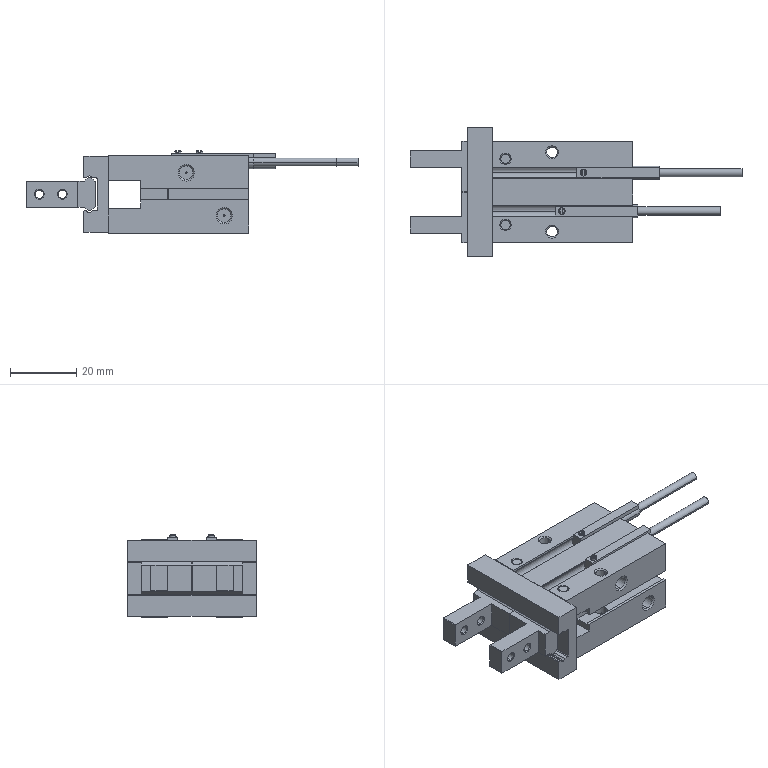Part | SolidWorks | 5 solids | 301 faces | box 100.5 x 39 x 24.85 mm | volume 31183 mm3 | plane 140 | cylinder 85 | cone 76 | commonest cylinder face diameters 3.242 x16 0.4 x10 2 x8 2.459 x8 1 x6 4 x6